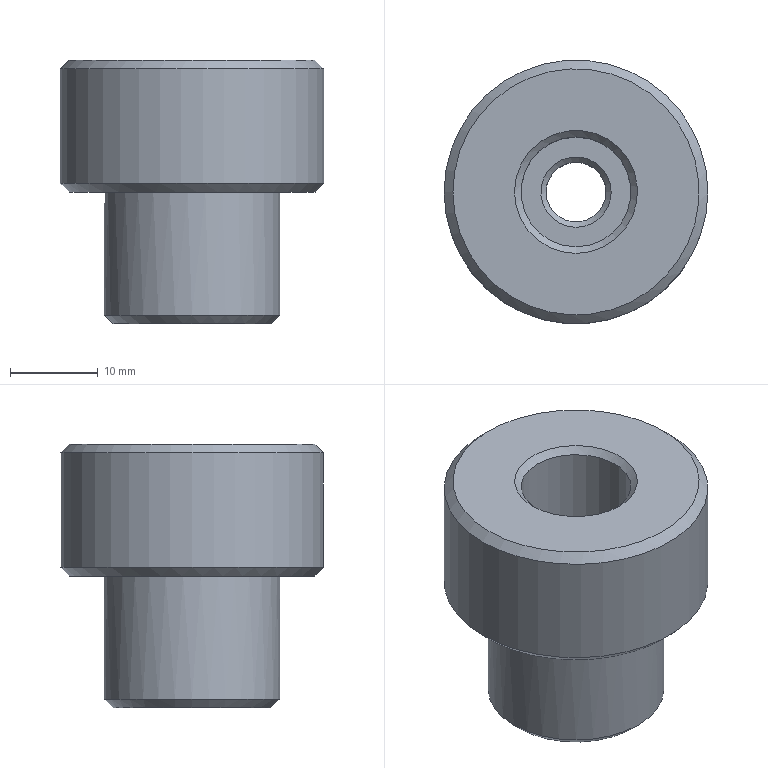Part | STEP file | 冲床-300配套压波_id538_x_t | 1 solid | 14 faces | box 30 x 30 x 30 mm | volume 12788 mm3 | cone 6 | plane 4 | cylinder 4 | commonest cylinder face diameters 6.8 x1 12.5 x1 20 x1 30 x1
STEP:
#1=CARTESIAN_POINT('',(1805.,-4.,183.));
#2=VERTEX_POINT('',#1);
#3=CARTESIAN_POINT('',(1805.,0.,183.));
#4=DIRECTION('',(0.,0.,-1.));
#5=DIRECTION('',(0.,-1.,0.));
#6=AXIS2_PLACEMENT_3D('',#3,#4,#5);
#7=CIRCLE('',#6,4.);
#8=EDGE_CURVE('',#2,#2,#7,.T.);
#9=ORIENTED_EDGE('',*,*,#8,.T.);
#10=EDGE_LOOP('',(#9));
#11=FACE_BOUND('',#10,.T.);
#12=CARTESIAN_POINT('',(1805.,-6.25,183.));
#13=VERTEX_POINT('',#12);
#14=CARTESIAN_POINT('',(1805.,0.,183.));
#15=DIRECTION('',(0.,0.,1.));
#16=DIRECTION('',(0.,-1.,0.));
#17=AXIS2_PLACEMENT_3D('',#14,#15,#16);
#18=CIRCLE('',#17,6.25);
#19=EDGE_CURVE('',#13,#13,#18,.T.);
#20=ORIENTED_EDGE('',*,*,#19,.T.);
#21=EDGE_LOOP('',(#20));
#22=FACE_BOUND('',#21,.T.);
#23=CARTESIAN_POINT('',(1805.,0.,183.));
#24=DIRECTION('',(0.,0.,1.));
#25=DIRECTION('',(-1.,0.,0.));
#26=AXIS2_PLACEMENT_3D('',#23,#24,#25);
#27=PLANE('',#26);
#28=ADVANCED_FACE('',(#11,#22),#27,.T.);
#29=CARTESIAN_POINT('',(1808.4,0.,182.4));
#30=VERTEX_POINT('',#29);
#31=CARTESIAN_POINT('',(1805.,0.,182.4));
#32=DIRECTION('',(0.,0.,1.));
#33=DIRECTION('',(1.,0.,0.));
#34=AXIS2_PLACEMENT_3D('',#31,#32,#33);
#35=CIRCLE('',#34,3.4);
#36=EDGE_CURVE('',#30,#30,#35,.T.);
#37=ORIENTED_EDGE('',*,*,#36,.T.);
#38=EDGE_LOOP('',(#37));
#39=FACE_BOUND('',#38,.T.);
#40=CARTESIAN_POINT('',(1801.6,0.,168.6));
#41=VERTEX_POINT('',#40);
#42=CARTESIAN_POINT('',(1805.,0.,168.6));
#43=DIRECTION('',(0.,0.,-1.));
#44=DIRECTION('',(-1.,0.,0.));
#45=AXIS2_PLACEMENT_3D('',#42,#43,#44);
#46=CIRCLE('',#45,3.4);
#47=EDGE_CURVE('',#41,#41,#46,.T.);
#48=ORIENTED_EDGE('',*,*,#47,.T.);
#49=EDGE_LOOP('',(#48));
#50=FACE_BOUND('',#49,.T.);
#51=CARTESIAN_POINT('',(1805.,0.,168.));
#52=DIRECTION('',(0.,0.,1.));
#53=DIRECTION('',(1.,0.,0.));
#54=AXIS2_PLACEMENT_3D('',#51,#52,#53);
#55=CYLINDRICAL_SURFACE('',#54,3.4);
#56=ADVANCED_FACE('',(#39,#50),#55,.F.);
#57=CARTESIAN_POINT('',(1798.,0.,198.));
#58=VERTEX_POINT('',#57);
#59=CARTESIAN_POINT('',(1805.,0.,198.));
#60=DIRECTION('',(0.,0.,-1.));
#61=DIRECTION('',(-1.,0.,0.));
#62=AXIS2_PLACEMENT_3D('',#59,#60,#61);
#63=CIRCLE('',#62,7.);
#64=EDGE_CURVE('',#58,#58,#63,.T.);
#65=ORIENTED_EDGE('',*,*,#64,.T.);
#66=EDGE_LOOP('',(#65));
#67=FACE_BOUND('',#66,.T.);
#68=CARTESIAN_POINT('',(1791.,0.,198.));
#69=VERTEX_POINT('',#68);
#70=CARTESIAN_POINT('',(1805.,0.,198.));
#71=DIRECTION('',(0.,0.,1.));
#72=DIRECTION('',(-1.,0.,0.));
#73=AXIS2_PLACEMENT_3D('',#70,#71,#72);
#74=CIRCLE('',#73,14.);
#75=EDGE_CURVE('',#69,#69,#74,.T.);
#76=ORIENTED_EDGE('',*,*,#75,.T.);
#77=EDGE_LOOP('',(#76));
#78=FACE_BOUND('',#77,.T.);
#79=CARTESIAN_POINT('',(1805.,0.,198.));
#80=DIRECTION('',(0.,0.,-1.));
#81=DIRECTION('',(-1.,0.,0.));
#82=AXIS2_PLACEMENT_3D('',#79,#80,#81);
#83=PLANE('',#82);
#84=ADVANCED_FACE('',(#67,#78),#83,.F.);
#85=CARTESIAN_POINT('',(1820.,0.,184.));
#86=VERTEX_POINT('',#85);
#87=CARTESIAN_POINT('',(1805.,0.,184.));
#88=DIRECTION('',(0.,0.,1.));
#89=DIRECTION('',(1.,0.,0.));
#90=AXIS2_PLACEMENT_3D('',#87,#88,#89);
#91=CIRCLE('',#90,15.);
#92=EDGE_CURVE('',#86,#86,#91,.T.);
#93=ORIENTED_EDGE('',*,*,#92,.T.);
#94=EDGE_LOOP('',(#93));
#95=FACE_BOUND('',#94,.T.);
#96=CARTESIAN_POINT('',(1790.,0.,197.));
#97=VERTEX_POINT('',#96);
#98=CARTESIAN_POINT('',(1805.,0.,197.));
#99=DIRECTION('',(0.,0.,-1.));
#100=DIRECTION('',(-1.,0.,0.));
#101=AXIS2_PLACEMENT_3D('',#98,#99,#100);
#102=CIRCLE('',#101,15.);
#103=EDGE_CURVE('',#97,#97,#102,.T.);
#104=ORIENTED_EDGE('',*,*,#103,.T.);
#105=EDGE_LOOP('',(#104));
#106=FACE_BOUND('',#105,.T.);
#107=CARTESIAN_POINT('',(1805.,0.,168.));
#108=DIRECTION('',(0.,0.,1.));
#109=DIRECTION('',(1.,0.,0.));
#110=AXIS2_PLACEMENT_3D('',#107,#108,#109);
#111=CYLINDRICAL_SURFACE('',#110,15.);
#112=ADVANCED_FACE('',(#95,#106),#111,.T.);
#113=CARTESIAN_POINT('',(1819.,0.,183.));
#114=VERTEX_POINT('',#113);
#115=CARTESIAN_POINT('',(1805.,0.,183.));
#116=DIRECTION('',(0.,0.,-1.));
#117=DIRECTION('',(1.,0.,0.));
#118=AXIS2_PLACEMENT_3D('',#115,#116,#117);
#119=CIRCLE('',#118,14.);
#120=EDGE_CURVE('',#114,#114,#119,.T.);
#121=ORIENTED_EDGE('',*,*,#120,.T.);
#122=EDGE_LOOP('',(#121));
#123=FACE_BOUND('',#122,.T.);
#124=CARTESIAN_POINT('',(1815.,0.,183.));
#125=VERTEX_POINT('',#124);
#126=CARTESIAN_POINT('',(1805.,0.,183.));
#127=DIRECTION('',(0.,0.,-1.));
#128=DIRECTION('',(1.,0.,0.));
#129=AXIS2_PLACEMENT_3D('',#126,#127,#128);
#130=CIRCLE('',#129,10.);
#131=EDGE_CURVE('',#125,#125,#130,.T.);
#132=ORIENTED_EDGE('',*,*,#131,.F.);
#133=EDGE_LOOP('',(#132));
#134=FACE_BOUND('',#133,.T.);
#135=CARTESIAN_POINT('',(1805.,0.,183.));
#136=DIRECTION('',(0.,0.,1.));
#137=DIRECTION('',(1.,0.,0.));
#138=AXIS2_PLACEMENT_3D('',#135,#136,#137);
#139=PLANE('',#138);
#140=ADVANCED_FACE('',(#123,#134),#139,.F.);
#141=CARTESIAN_POINT('',(1795.,0.,169.));
#142=VERTEX_POINT('',#141);
#143=CARTESIAN_POINT('',(1805.,0.,169.));
#144=DIRECTION('',(0.,0.,1.));
#145=DIRECTION('',(-1.,0.,0.));
#146=AXIS2_PLACEMENT_3D('',#143,#144,#145);
#147=CIRCLE('',#146,10.);
#148=EDGE_CURVE('',#142,#142,#147,.T.);
#149=ORIENTED_EDGE('',*,*,#148,.T.);
#150=EDGE_LOOP('',(#149));
#151=FACE_BOUND('',#150,.T.);
#152=ORIENTED_EDGE('',*,*,#131,.T.);
#153=EDGE_LOOP('',(#152));
#154=FACE_BOUND('',#153,.T.);
#155=CARTESIAN_POINT('',(1805.,0.,168.));
#156=DIRECTION('',(0.,0.,1.));
#157=DIRECTION('',(1.,0.,0.));
#158=AXIS2_PLACEMENT_3D('',#155,#156,#157);
#159=CYLINDRICAL_SURFACE('',#158,10.);
#160=ADVANCED_FACE('',(#151,#154),#159,.T.);
#161=CARTESIAN_POINT('',(1801.,0.,168.));
#162=VERTEX_POINT('',#161);
#163=CARTESIAN_POINT('',(1805.,0.,168.));
#164=DIRECTION('',(0.,0.,1.));
#165=DIRECTION('',(-1.,0.,0.));
#166=AXIS2_PLACEMENT_3D('',#163,#164,#165);
#167=CIRCLE('',#166,4.);
#168=EDGE_CURVE('',#162,#162,#167,.T.);
#169=ORIENTED_EDGE('',*,*,#168,.T.);
#170=EDGE_LOOP('',(#169));
#171=FACE_BOUND('',#170,.T.);
#172=CARTESIAN_POINT('',(1796.,0.,168.));
#173=VERTEX_POINT('',#172);
#174=CARTESIAN_POINT('',(1805.,0.,168.));
#175=DIRECTION('',(0.,0.,-1.));
#176=DIRECTION('',(-1.,0.,0.));
#177=AXIS2_PLACEMENT_3D('',#174,#175,#176);
#178=CIRCLE('',#177,9.);
#179=EDGE_CURVE('',#173,#173,#178,.T.);
#180=ORIENTED_EDGE('',*,*,#179,.T.);
#181=EDGE_LOOP('',(#180));
#182=FACE_BOUND('',#181,.T.);
#183=CARTESIAN_POINT('',(1805.,0.,168.));
#184=DIRECTION('',(0.,0.,-1.));
#185=DIRECTION('',(-1.,0.,0.));
#186=AXIS2_PLACEMENT_3D('',#183,#184,#185);
#187=PLANE('',#186);
#188=ADVANCED_FACE('',(#171,#182),#187,.T.);
#189=ORIENTED_EDGE('',*,*,#148,.F.);
#190=EDGE_LOOP('',(#189));
#191=FACE_BOUND('',#190,.T.);
#192=ORIENTED_EDGE('',*,*,#179,.F.);
#193=EDGE_LOOP('',(#192));
#194=FACE_BOUND('',#193,.T.);
#195=CARTESIAN_POINT('',(1805.,0.,168.));
#196=DIRECTION('',(0.,0.,1.));
#197=DIRECTION('',(1.,0.,0.));
#198=AXIS2_PLACEMENT_3D('',#195,#196,#197);
#199=CONICAL_SURFACE('',#198,9.,45.);
#200=ADVANCED_FACE('',(#191,#194),#199,.T.);
#201=ORIENTED_EDGE('',*,*,#120,.F.);
#202=EDGE_LOOP('',(#201));
#203=FACE_BOUND('',#202,.T.);
#204=ORIENTED_EDGE('',*,*,#92,.F.);
#205=EDGE_LOOP('',(#204));
#206=FACE_BOUND('',#205,.T.);
#207=CARTESIAN_POINT('',(1805.,0.,184.));
#208=DIRECTION('',(0.,0.,1.));
#209=DIRECTION('',(1.,0.,0.));
#210=AXIS2_PLACEMENT_3D('',#207,#208,#209);
#211=CONICAL_SURFACE('',#210,15.,45.);
#212=ADVANCED_FACE('',(#203,#206),#211,.T.);
#213=ORIENTED_EDGE('',*,*,#75,.F.);
#214=EDGE_LOOP('',(#213));
#215=FACE_BOUND('',#214,.T.);
#216=ORIENTED_EDGE('',*,*,#103,.F.);
#217=EDGE_LOOP('',(#216));
#218=FACE_BOUND('',#217,.T.);
#219=CARTESIAN_POINT('',(1805.,0.,197.));
#220=DIRECTION('',(0.,0.,-1.));
#221=DIRECTION('',(-1.,0.,0.));
#222=AXIS2_PLACEMENT_3D('',#219,#220,#221);
#223=CONICAL_SURFACE('',#222,15.,45.);
#224=ADVANCED_FACE('',(#215,#218),#223,.T.);
#225=ORIENTED_EDGE('',*,*,#47,.F.);
#226=EDGE_LOOP('',(#225));
#227=FACE_BOUND('',#226,.T.);
#228=ORIENTED_EDGE('',*,*,#168,.F.);
#229=EDGE_LOOP('',(#228));
#230=FACE_BOUND('',#229,.T.);
#231=CARTESIAN_POINT('',(1805.,0.,168.));
#232=DIRECTION('',(0.,0.,-1.));
#233=DIRECTION('',(-1.,0.,0.));
#234=AXIS2_PLACEMENT_3D('',#231,#232,#233);
#235=CONICAL_SURFACE('',#234,4.,45.);
#236=ADVANCED_FACE('',(#227,#230),#235,.F.);
#237=CARTESIAN_POINT('',(1805.,6.25,197.25));
#238=VERTEX_POINT('',#237);
#239=CARTESIAN_POINT('',(1805.,0.,197.25));
#240=DIRECTION('',(0.,0.,1.));
#241=DIRECTION('',(0.,1.,0.));
#242=AXIS2_PLACEMENT_3D('',#239,#240,#241);
#243=CIRCLE('',#242,6.25);
#244=EDGE_CURVE('',#238,#238,#243,.T.);
#245=ORIENTED_EDGE('',*,*,#244,.T.);
#246=EDGE_LOOP('',(#245));
#247=FACE_BOUND('',#246,.T.);
#248=ORIENTED_EDGE('',*,*,#19,.F.);
#249=EDGE_LOOP('',(#248));
#250=FACE_BOUND('',#249,.T.);
#251=CARTESIAN_POINT('',(1805.,0.,211.));
#252=DIRECTION('',(0.,0.,-1.));
#253=DIRECTION('',(1.,0.,0.));
#254=AXIS2_PLACEMENT_3D('',#251,#252,#253);
#255=CYLINDRICAL_SURFACE('',#254,6.25);
#256=ADVANCED_FACE('',(#247,#250),#255,.F.);
#257=ORIENTED_EDGE('',*,*,#244,.F.);
#258=EDGE_LOOP('',(#257));
#259=FACE_BOUND('',#258,.T.);
#260=ORIENTED_EDGE('',*,*,#64,.F.);
#261=EDGE_LOOP('',(#260));
#262=FACE_BOUND('',#261,.T.);
#263=CARTESIAN_POINT('',(1805.,0.,198.));
#264=DIRECTION('',(0.,0.,1.));
#265=DIRECTION('',(0.,-1.,0.));
#266=AXIS2_PLACEMENT_3D('',#263,#264,#265);
#267=CONICAL_SURFACE('',#266,7.,45.);
#268=ADVANCED_FACE('',(#259,#262),#267,.F.);
#269=ORIENTED_EDGE('',*,*,#36,.F.);
#270=EDGE_LOOP('',(#269));
#271=FACE_BOUND('',#270,.T.);
#272=ORIENTED_EDGE('',*,*,#8,.F.);
#273=EDGE_LOOP('',(#272));
#274=FACE_BOUND('',#273,.T.);
#275=CARTESIAN_POINT('',(1805.,0.,183.));
#276=DIRECTION('',(0.,0.,1.));
#277=DIRECTION('',(1.,0.,0.));
#278=AXIS2_PLACEMENT_3D('',#275,#276,#277);
#279=CONICAL_SURFACE('',#278,4.,45.);
#280=ADVANCED_FACE('',(#271,#274),#279,.F.);
#281=CLOSED_SHELL('',(#28,#56,#84,#112,#140,#160,#188,#200,#212,#224,#236,#256,#268,#280));
#282=MANIFOLD_SOLID_BREP('',#281);
#283=(LENGTH_UNIT()NAMED_UNIT(*)SI_UNIT(.MILLI.,.METRE.));
#284=UNCERTAINTY_MEASURE_WITH_UNIT(LENGTH_MEASURE(0.00002),#283,'','');
#285=(NAMED_UNIT(*)PLANE_ANGLE_UNIT()SI_UNIT($,.RADIAN.));
#286=PLANE_ANGLE_MEASURE_WITH_UNIT(PLANE_ANGLE_MEASURE(0.01745),#285);
#287=DIMENSIONAL_EXPONENTS(0.,0.,0.,0.,0.,0.,0.);
#288=(CONVERSION_BASED_UNIT('DEGREE',#286)NAMED_UNIT(#287)PLANE_ANGLE_UNIT());
#289=(NAMED_UNIT(*)SI_UNIT($,.STERADIAN.)SOLID_ANGLE_UNIT());
#290=(GEOMETRIC_REPRESENTATION_CONTEXT(3)GLOBAL_UNCERTAINTY_ASSIGNED_CONTEXT((#284))GLOBAL_UNIT_ASSIGNED_CONTEXT((#283,#288,#289))REPRESENTATION_CONTEXT('',''));
#291=ADVANCED_BREP_SHAPE_REPRESENTATION('',(#282),#290);